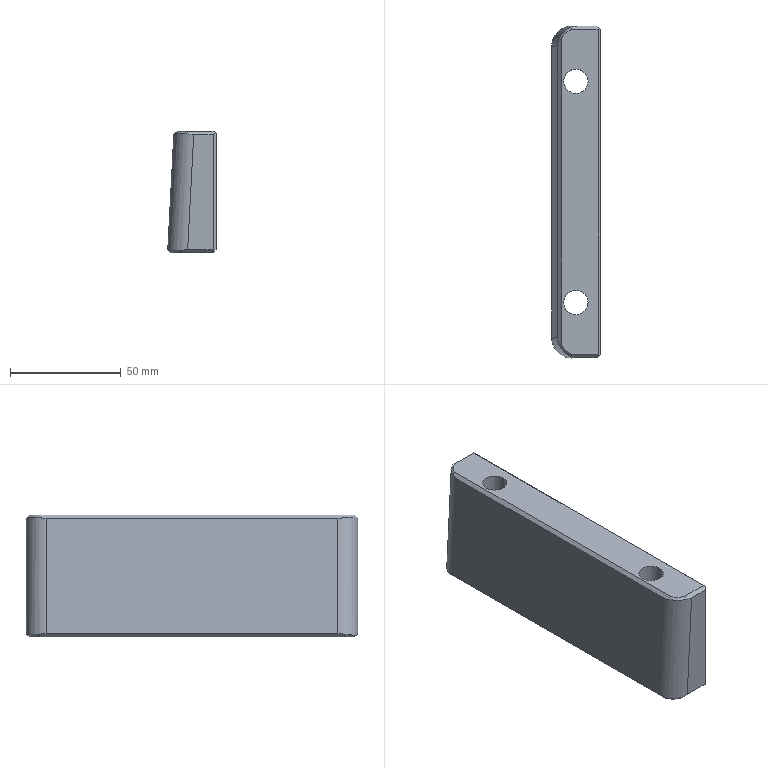Part | Creo | 1 solid | 39 faces | box 21.922 x 150 x 55 mm | volume 149569 mm3 | plane 19 | cylinder 14 | spline 4 | cone 2 | commonest cylinder face diameters 18 x6 11 x4 8.5 x2 10 x2
STEP:
#1=CARTESIAN_POINT('',(-140.,-145.005,33.5));
#2=VERTEX_POINT('',#1);
#3=CARTESIAN_POINT('',(-122.,-145.005,33.5));
#4=VERTEX_POINT('',#3);
#5=CARTESIAN_POINT('',(-131.,-145.005,33.5));
#6=DIRECTION('',(0.,0.,1.));
#7=DIRECTION('',(-1.,-0.000000059,0.));
#8=AXIS2_PLACEMENT_3D('',#5,#6,#7);
#9=CIRCLE('',#8,9.);
#10=EDGE_CURVE('',#2,#4,#9,.T.);
#11=ORIENTED_EDGE('',*,*,#10,.T.);
#12=CARTESIAN_POINT('',(-122.,-145.005,49.5));
#13=VERTEX_POINT('',#12);
#14=CARTESIAN_POINT('',(-122.,-145.005,33.5));
#15=DIRECTION('',(0.,-0.000000011,1.));
#16=VECTOR('',#15,16.);
#17=LINE('',#14,#16);
#18=EDGE_CURVE('',#4,#13,#17,.T.);
#19=ORIENTED_EDGE('',*,*,#18,.T.);
#20=CARTESIAN_POINT('',(-140.,-145.005,49.5));
#21=VERTEX_POINT('',#20);
#22=CARTESIAN_POINT('',(-131.,-145.005,49.5));
#23=DIRECTION('',(0.,0.,-1.));
#24=DIRECTION('',(1.,0.,0.));
#25=AXIS2_PLACEMENT_3D('',#22,#23,#24);
#26=CIRCLE('',#25,9.);
#27=EDGE_CURVE('',#13,#21,#26,.T.);
#28=ORIENTED_EDGE('',*,*,#27,.T.);
#29=CARTESIAN_POINT('',(-140.,-145.005,33.5));
#30=DIRECTION('',(0.,0.,1.));
#31=VECTOR('',#30,16.);
#32=LINE('',#29,#31);
#33=EDGE_CURVE('',#2,#21,#32,.T.);
#34=ORIENTED_EDGE('',*,*,#33,.F.);
#35=EDGE_LOOP('',(#11,#19,#28,#34));
#36=FACE_OUTER_BOUND('',#35,.F.);
#37=CARTESIAN_POINT('',(-131.,-145.005,32.95));
#38=DIRECTION('',(0.,0.,1.));
#39=DIRECTION('',(-1.,-0.000000059,0.));
#40=AXIS2_PLACEMENT_3D('',#37,#38,#39);
#41=CYLINDRICAL_SURFACE('',#40,9.);
#42=ADVANCED_FACE('',(#36),#41,.F.);
#43=CARTESIAN_POINT('',(-140.5,-163.758,33.5));
#44=VERTEX_POINT('',#43);
#45=CARTESIAN_POINT('',(-140.5,-26.251,33.5));
#46=VERTEX_POINT('',#45);
#47=CARTESIAN_POINT('',(-140.5,-163.758,33.5));
#48=DIRECTION('',(-0.000000059,1.,0.));
#49=VECTOR('',#48,137.507);
#50=LINE('',#47,#49);
#51=EDGE_CURVE('',#44,#46,#50,.T.);
#52=ORIENTED_EDGE('',*,*,#51,.F.);
#53=CARTESIAN_POINT('',(-135.628,-168.581,33.5));
#54=VERTEX_POINT('',#53);
#55=CARTESIAN_POINT('',(-135.628,-168.581,33.5));
#56=CARTESIAN_POINT('',(-137.859,-167.798,33.5));
#57=CARTESIAN_POINT('',(-139.697,-165.98,33.5));
#58=CARTESIAN_POINT('',(-140.5,-163.758,33.5));
#59=B_SPLINE_CURVE_WITH_KNOTS('',3,(#55,#56,#57,#58),.UNSPECIFIED.,.F.,.F.,(4,4),(0.,1.),.UNSPECIFIED.);
#60=EDGE_CURVE('',#54,#44,#59,.T.);
#61=ORIENTED_EDGE('',*,*,#60,.F.);
#62=CARTESIAN_POINT('',(-121.423,-168.581,33.5));
#63=VERTEX_POINT('',#62);
#64=CARTESIAN_POINT('',(-121.423,-168.581,33.5));
#65=DIRECTION('',(-1.,-0.000000062,-0.000000002));
#66=VECTOR('',#65,14.205);
#67=LINE('',#64,#66);
#68=EDGE_CURVE('',#63,#54,#67,.T.);
#69=ORIENTED_EDGE('',*,*,#68,.F.);
#70=CARTESIAN_POINT('',(-121.423,-21.428,33.5));
#71=VERTEX_POINT('',#70);
#72=CARTESIAN_POINT('',(-121.423,-21.428,33.5));
#73=DIRECTION('',(0.000000059,-1.,0.));
#74=VECTOR('',#73,147.153);
#75=LINE('',#72,#74);
#76=EDGE_CURVE('',#71,#63,#75,.T.);
#77=ORIENTED_EDGE('',*,*,#76,.F.);
#78=CARTESIAN_POINT('',(-135.628,-21.428,33.5));
#79=VERTEX_POINT('',#78);
#80=CARTESIAN_POINT('',(-135.628,-21.428,33.5));
#81=DIRECTION('',(1.,0.000000059,0.));
#82=VECTOR('',#81,14.205);
#83=LINE('',#80,#82);
#84=EDGE_CURVE('',#79,#71,#83,.T.);
#85=ORIENTED_EDGE('',*,*,#84,.F.);
#86=CARTESIAN_POINT('',(-140.5,-26.251,33.5));
#87=CARTESIAN_POINT('',(-139.697,-24.029,33.5));
#88=CARTESIAN_POINT('',(-137.859,-22.211,33.5));
#89=B_SPLINE_CURVE_WITH_KNOTS('',3,(#86,#87,#88,#78),.UNSPECIFIED.,.F.,.F.,(4,4),(0.,1.),.UNSPECIFIED.);
#90=EDGE_CURVE('',#46,#79,#89,.T.);
#91=ORIENTED_EDGE('',*,*,#90,.F.);
#92=EDGE_LOOP('',(#52,#61,#69,#77,#85,#91));
#93=FACE_OUTER_BOUND('',#92,.F.);
#94=CARTESIAN_POINT('',(-140.,-45.005,33.5));
#95=VERTEX_POINT('',#94);
#96=CARTESIAN_POINT('',(-122.,-45.005,33.5));
#97=VERTEX_POINT('',#96);
#98=CARTESIAN_POINT('',(-131.,-45.005,33.5));
#99=DIRECTION('',(0.,0.,1.));
#100=DIRECTION('',(-1.,-0.000000059,0.));
#101=AXIS2_PLACEMENT_3D('',#98,#99,#100);
#102=CIRCLE('',#101,9.);
#103=EDGE_CURVE('',#95,#97,#102,.T.);
#104=ORIENTED_EDGE('',*,*,#103,.F.);
#105=CARTESIAN_POINT('',(-131.,-45.005,33.5));
#106=DIRECTION('',(0.,0.,1.));
#107=DIRECTION('',(1.,0.000000059,0.));
#108=AXIS2_PLACEMENT_3D('',#105,#106,#107);
#109=CIRCLE('',#108,9.);
#110=EDGE_CURVE('',#97,#95,#109,.T.);
#111=ORIENTED_EDGE('',*,*,#110,.F.);
#112=EDGE_LOOP('',(#104,#111));
#113=FACE_BOUND('',#112,.F.);
#114=ORIENTED_EDGE('',*,*,#10,.F.);
#115=CARTESIAN_POINT('',(-131.,-145.005,33.5));
#116=DIRECTION('',(0.,0.,1.));
#117=DIRECTION('',(1.,0.000000059,0.));
#118=AXIS2_PLACEMENT_3D('',#115,#116,#117);
#119=CIRCLE('',#118,9.);
#120=EDGE_CURVE('',#4,#2,#119,.T.);
#121=ORIENTED_EDGE('',*,*,#120,.F.);
#122=EDGE_LOOP('',(#114,#121));
#123=FACE_BOUND('',#122,.F.);
#124=CARTESIAN_POINT('',(-126.,-95.005,33.5));
#125=VERTEX_POINT('',#124);
#126=CARTESIAN_POINT('',(-136.,-95.005,33.5));
#127=VERTEX_POINT('',#126);
#128=CARTESIAN_POINT('',(-131.,-95.005,33.5));
#129=DIRECTION('',(0.,0.,1.));
#130=DIRECTION('',(1.,0.,0.));
#131=AXIS2_PLACEMENT_3D('',#128,#129,#130);
#132=CIRCLE('',#131,5.);
#133=EDGE_CURVE('',#125,#127,#132,.T.);
#134=ORIENTED_EDGE('',*,*,#133,.F.);
#135=CARTESIAN_POINT('',(-131.,-95.005,33.5));
#136=DIRECTION('',(0.,0.,1.));
#137=DIRECTION('',(-1.,0.,0.));
#138=AXIS2_PLACEMENT_3D('',#135,#136,#137);
#139=CIRCLE('',#138,5.);
#140=EDGE_CURVE('',#127,#125,#139,.T.);
#141=ORIENTED_EDGE('',*,*,#140,.F.);
#142=EDGE_LOOP('',(#134,#141));
#143=FACE_BOUND('',#142,.F.);
#144=CARTESIAN_POINT('',(-142.,-20.005,33.5));
#145=DIRECTION('',(0.,0.,-1.));
#146=DIRECTION('',(1.,0.000000059,0.));
#147=AXIS2_PLACEMENT_3D('',#144,#145,#146);
#148=PLANE('',#147);
#149=ADVANCED_FACE('',(#93,#113,#123,#143),#148,.T.);
#150=ORIENTED_EDGE('',*,*,#120,.T.);
#151=ORIENTED_EDGE('',*,*,#33,.T.);
#152=CARTESIAN_POINT('',(-131.,-145.005,49.5));
#153=DIRECTION('',(0.,0.,-1.));
#154=DIRECTION('',(-1.,-0.000000059,0.));
#155=AXIS2_PLACEMENT_3D('',#152,#153,#154);
#156=CIRCLE('',#155,9.);
#157=EDGE_CURVE('',#21,#13,#156,.T.);
#158=ORIENTED_EDGE('',*,*,#157,.T.);
#159=ORIENTED_EDGE('',*,*,#18,.F.);
#160=EDGE_LOOP('',(#150,#151,#158,#159));
#161=FACE_OUTER_BOUND('',#160,.F.);
#162=CARTESIAN_POINT('',(-131.,-145.005,32.95));
#163=DIRECTION('',(0.,0.,1.));
#164=DIRECTION('',(-1.,-0.000000059,0.));
#165=AXIS2_PLACEMENT_3D('',#162,#163,#164);
#166=CYLINDRICAL_SURFACE('',#165,9.);
#167=ADVANCED_FACE('',(#161),#166,.F.);
#168=ORIENTED_EDGE('',*,*,#27,.F.);
#169=ORIENTED_EDGE('',*,*,#157,.F.);
#170=EDGE_LOOP('',(#168,#169));
#171=FACE_OUTER_BOUND('',#170,.F.);
#172=CARTESIAN_POINT('',(-125.5,-145.005,49.5));
#173=VERTEX_POINT('',#172);
#174=CARTESIAN_POINT('',(-136.5,-145.005,49.5));
#175=VERTEX_POINT('',#174);
#176=CARTESIAN_POINT('',(-131.,-145.005,49.5));
#177=DIRECTION('',(0.,0.,1.));
#178=DIRECTION('',(1.,0.,0.));
#179=AXIS2_PLACEMENT_3D('',#176,#177,#178);
#180=CIRCLE('',#179,5.5);
#181=EDGE_CURVE('',#173,#175,#180,.T.);
#182=ORIENTED_EDGE('',*,*,#181,.F.);
#183=CARTESIAN_POINT('',(-131.,-145.005,49.5));
#184=DIRECTION('',(0.,0.,1.));
#185=DIRECTION('',(-1.,-0.000000059,0.));
#186=AXIS2_PLACEMENT_3D('',#183,#184,#185);
#187=CIRCLE('',#186,5.5);
#188=EDGE_CURVE('',#175,#173,#187,.T.);
#189=ORIENTED_EDGE('',*,*,#188,.F.);
#190=EDGE_LOOP('',(#182,#189));
#191=FACE_BOUND('',#190,.F.);
#192=CARTESIAN_POINT('',(-131.,-145.005,49.5));
#193=DIRECTION('',(0.,0.,1.));
#194=DIRECTION('',(-1.,-0.000000059,0.));
#195=AXIS2_PLACEMENT_3D('',#192,#193,#194);
#196=PLANE('',#195);
#197=ADVANCED_FACE('',(#171,#191),#196,.F.);
#198=ORIENTED_EDGE('',*,*,#181,.T.);
#199=CARTESIAN_POINT('',(-136.5,-145.005,88.5));
#200=VERTEX_POINT('',#199);
#201=CARTESIAN_POINT('',(-136.5,-145.005,88.5));
#202=DIRECTION('',(0.,0.,-1.));
#203=VECTOR('',#202,39.);
#204=LINE('',#201,#203);
#205=EDGE_CURVE('',#200,#175,#204,.T.);
#206=ORIENTED_EDGE('',*,*,#205,.F.);
#207=CARTESIAN_POINT('',(-125.5,-145.005,88.5));
#208=VERTEX_POINT('',#207);
#209=CARTESIAN_POINT('',(-131.,-145.005,88.5));
#210=DIRECTION('',(0.,0.,-1.));
#211=DIRECTION('',(-1.,-0.000000059,0.));
#212=AXIS2_PLACEMENT_3D('',#209,#210,#211);
#213=CIRCLE('',#212,5.5);
#214=EDGE_CURVE('',#200,#208,#213,.T.);
#215=ORIENTED_EDGE('',*,*,#214,.T.);
#216=CARTESIAN_POINT('',(-125.5,-145.005,88.5));
#217=DIRECTION('',(0.,-0.000000003,-1.));
#218=VECTOR('',#217,39.);
#219=LINE('',#216,#218);
#220=EDGE_CURVE('',#208,#173,#219,.T.);
#221=ORIENTED_EDGE('',*,*,#220,.T.);
#222=EDGE_LOOP('',(#198,#206,#215,#221));
#223=FACE_OUTER_BOUND('',#222,.F.);
#224=CARTESIAN_POINT('',(-131.,-145.005,44.5));
#225=DIRECTION('',(0.,0.,-1.));
#226=DIRECTION('',(-1.,-0.000000059,0.));
#227=AXIS2_PLACEMENT_3D('',#224,#225,#226);
#228=CYLINDRICAL_SURFACE('',#227,5.5);
#229=ADVANCED_FACE('',(#223),#228,.F.);
#230=ORIENTED_EDGE('',*,*,#188,.T.);
#231=ORIENTED_EDGE('',*,*,#220,.F.);
#232=CARTESIAN_POINT('',(-131.,-145.005,88.5));
#233=DIRECTION('',(0.,0.,-1.));
#234=DIRECTION('',(1.,0.000000059,0.));
#235=AXIS2_PLACEMENT_3D('',#232,#233,#234);
#236=CIRCLE('',#235,5.5);
#237=EDGE_CURVE('',#208,#200,#236,.T.);
#238=ORIENTED_EDGE('',*,*,#237,.T.);
#239=ORIENTED_EDGE('',*,*,#205,.T.);
#240=EDGE_LOOP('',(#230,#231,#238,#239));
#241=FACE_OUTER_BOUND('',#240,.F.);
#242=CARTESIAN_POINT('',(-131.,-145.005,44.5));
#243=DIRECTION('',(0.,0.,-1.));
#244=DIRECTION('',(-1.,-0.000000059,0.));
#245=AXIS2_PLACEMENT_3D('',#242,#243,#244);
#246=CYLINDRICAL_SURFACE('',#245,5.5);
#247=ADVANCED_FACE('',(#241),#246,.F.);
#248=CARTESIAN_POINT('',(-121.,-21.585,88.5));
#249=VERTEX_POINT('',#248);
#250=CARTESIAN_POINT('',(-133.06,-21.585,88.5));
#251=VERTEX_POINT('',#250);
#252=CARTESIAN_POINT('',(-121.,-21.585,88.5));
#253=DIRECTION('',(-1.,-0.000000052,0.000000002));
#254=VECTOR('',#253,12.06);
#255=LINE('',#252,#254);
#256=EDGE_CURVE('',#249,#251,#255,.T.);
#257=ORIENTED_EDGE('',*,*,#256,.F.);
#258=CARTESIAN_POINT('',(-121.,-168.424,88.5));
#259=VERTEX_POINT('',#258);
#260=CARTESIAN_POINT('',(-121.,-21.585,88.5));
#261=DIRECTION('',(0.000000059,-1.,0.));
#262=VECTOR('',#261,146.839);
#263=LINE('',#260,#262);
#264=EDGE_CURVE('',#249,#259,#263,.T.);
#265=ORIENTED_EDGE('',*,*,#264,.T.);
#266=CARTESIAN_POINT('',(-133.06,-168.424,88.5));
#267=VERTEX_POINT('',#266);
#268=CARTESIAN_POINT('',(-133.06,-168.424,88.5));
#269=DIRECTION('',(1.,0.000000059,0.));
#270=VECTOR('',#269,12.06);
#271=LINE('',#268,#270);
#272=EDGE_CURVE('',#267,#259,#271,.T.);
#273=ORIENTED_EDGE('',*,*,#272,.F.);
#274=CARTESIAN_POINT('',(-137.618,-163.828,88.5));
#275=VERTEX_POINT('',#274);
#276=CARTESIAN_POINT('',(-137.618,-163.828,88.5));
#277=CARTESIAN_POINT('',(-136.834,-165.908,88.5));
#278=CARTESIAN_POINT('',(-135.136,-167.622,88.5));
#279=B_SPLINE_CURVE_WITH_KNOTS('',3,(#276,#277,#278,#266),.UNSPECIFIED.,.F.,.F.,(4,4),(0.,1.),.UNSPECIFIED.);
#280=EDGE_CURVE('',#275,#267,#279,.T.);
#281=ORIENTED_EDGE('',*,*,#280,.F.);
#282=CARTESIAN_POINT('',(-137.618,-26.182,88.5));
#283=VERTEX_POINT('',#282);
#284=CARTESIAN_POINT('',(-137.618,-26.182,88.5));
#285=DIRECTION('',(0.000000058,-1.,0.));
#286=VECTOR('',#285,137.646);
#287=LINE('',#284,#286);
#288=EDGE_CURVE('',#283,#275,#287,.T.);
#289=ORIENTED_EDGE('',*,*,#288,.F.);
#290=CARTESIAN_POINT('',(-133.06,-21.585,88.5));
#291=CARTESIAN_POINT('',(-135.136,-22.388,88.5));
#292=CARTESIAN_POINT('',(-136.834,-24.101,88.5));
#293=B_SPLINE_CURVE_WITH_KNOTS('',3,(#290,#291,#292,#282),.UNSPECIFIED.,.F.,.F.,(4,4),(0.,1.),.UNSPECIFIED.);
#294=EDGE_CURVE('',#251,#283,#293,.T.);
#295=ORIENTED_EDGE('',*,*,#294,.F.);
#296=EDGE_LOOP('',(#257,#265,#273,#281,#289,#295));
#297=FACE_OUTER_BOUND('',#296,.F.);
#298=CARTESIAN_POINT('',(-136.5,-45.005,88.5));
#299=VERTEX_POINT('',#298);
#300=CARTESIAN_POINT('',(-125.5,-45.005,88.5));
#301=VERTEX_POINT('',#300);
#302=CARTESIAN_POINT('',(-131.,-45.005,88.5));
#303=DIRECTION('',(0.,0.,-1.));
#304=DIRECTION('',(-1.,-0.000000059,0.));
#305=AXIS2_PLACEMENT_3D('',#302,#303,#304);
#306=CIRCLE('',#305,5.5);
#307=EDGE_CURVE('',#299,#301,#306,.T.);
#308=ORIENTED_EDGE('',*,*,#307,.F.);
#309=CARTESIAN_POINT('',(-131.,-45.005,88.5));
#310=DIRECTION('',(0.,0.,-1.));
#311=DIRECTION('',(1.,0.000000059,0.));
#312=AXIS2_PLACEMENT_3D('',#309,#310,#311);
#313=CIRCLE('',#312,5.5);
#314=EDGE_CURVE('',#301,#299,#313,.T.);
#315=ORIENTED_EDGE('',*,*,#314,.F.);
#316=EDGE_LOOP('',(#308,#315));
#317=FACE_BOUND('',#316,.F.);
#318=ORIENTED_EDGE('',*,*,#214,.F.);
#319=ORIENTED_EDGE('',*,*,#237,.F.);
#320=EDGE_LOOP('',(#318,#319));
#321=FACE_BOUND('',#320,.F.);
#322=CARTESIAN_POINT('',(-120.,-20.005,88.5));
#323=DIRECTION('',(0.,0.,1.));
#324=DIRECTION('',(-1.,-0.000000059,0.));
#325=AXIS2_PLACEMENT_3D('',#322,#323,#324);
#326=PLANE('',#325);
#327=ADVANCED_FACE('',(#297,#317,#321),#326,.T.);
#328=CARTESIAN_POINT('',(-125.5,-45.005,49.5));
#329=VERTEX_POINT('',#328);
#330=CARTESIAN_POINT('',(-136.5,-45.005,49.5));
#331=VERTEX_POINT('',#330);
#332=CARTESIAN_POINT('',(-131.,-45.005,49.5));
#333=DIRECTION('',(0.,0.,1.));
#334=DIRECTION('',(1.,0.,0.));
#335=AXIS2_PLACEMENT_3D('',#332,#333,#334);
#336=CIRCLE('',#335,5.5);
#337=EDGE_CURVE('',#329,#331,#336,.T.);
#338=ORIENTED_EDGE('',*,*,#337,.T.);
#339=CARTESIAN_POINT('',(-136.5,-45.005,88.5));
#340=DIRECTION('',(0.,0.,-1.));
#341=VECTOR('',#340,39.);
#342=LINE('',#339,#341);
#343=EDGE_CURVE('',#299,#331,#342,.T.);
#344=ORIENTED_EDGE('',*,*,#343,.F.);
#345=ORIENTED_EDGE('',*,*,#307,.T.);
#346=CARTESIAN_POINT('',(-125.5,-45.005,88.5));
#347=DIRECTION('',(0.,-0.000000003,-1.));
#348=VECTOR('',#347,39.);
#349=LINE('',#346,#348);
#350=EDGE_CURVE('',#301,#329,#349,.T.);
#351=ORIENTED_EDGE('',*,*,#350,.T.);
#352=EDGE_LOOP('',(#338,#344,#345,#351));
#353=FACE_OUTER_BOUND('',#352,.F.);
#354=CARTESIAN_POINT('',(-131.,-45.005,44.5));
#355=DIRECTION('',(0.,0.,-1.));
#356=DIRECTION('',(-1.,-0.000000059,0.));
#357=AXIS2_PLACEMENT_3D('',#354,#355,#356);
#358=CYLINDRICAL_SURFACE('',#357,5.5);
#359=ADVANCED_FACE('',(#353),#358,.F.);
#360=CARTESIAN_POINT('',(-122.,-45.005,49.5));
#361=VERTEX_POINT('',#360);
#362=CARTESIAN_POINT('',(-140.,-45.005,49.5));
#363=VERTEX_POINT('',#362);
#364=CARTESIAN_POINT('',(-131.,-45.005,49.5));
#365=DIRECTION('',(0.,0.,-1.));
#366=DIRECTION('',(1.,0.,0.));
#367=AXIS2_PLACEMENT_3D('',#364,#365,#366);
#368=CIRCLE('',#367,9.);
#369=EDGE_CURVE('',#361,#363,#368,.T.);
#370=ORIENTED_EDGE('',*,*,#369,.F.);
#371=CARTESIAN_POINT('',(-131.,-45.005,49.5));
#372=DIRECTION('',(0.,0.,-1.));
#373=DIRECTION('',(-1.,-0.000000059,0.));
#374=AXIS2_PLACEMENT_3D('',#371,#372,#373);
#375=CIRCLE('',#374,9.);
#376=EDGE_CURVE('',#363,#361,#375,.T.);
#377=ORIENTED_EDGE('',*,*,#376,.F.);
#378=EDGE_LOOP('',(#370,#377));
#379=FACE_OUTER_BOUND('',#378,.F.);
#380=ORIENTED_EDGE('',*,*,#337,.F.);
#381=CARTESIAN_POINT('',(-131.,-45.005,49.5));
#382=DIRECTION('',(0.,0.,1.));
#383=DIRECTION('',(-1.,-0.000000059,0.));
#384=AXIS2_PLACEMENT_3D('',#381,#382,#383);
#385=CIRCLE('',#384,5.5);
#386=EDGE_CURVE('',#331,#329,#385,.T.);
#387=ORIENTED_EDGE('',*,*,#386,.F.);
#388=EDGE_LOOP('',(#380,#387));
#389=FACE_BOUND('',#388,.F.);
#390=CARTESIAN_POINT('',(-131.,-45.005,49.5));
#391=DIRECTION('',(0.,0.,1.));
#392=DIRECTION('',(-1.,-0.000000059,0.));
#393=AXIS2_PLACEMENT_3D('',#390,#391,#392);
#394=PLANE('',#393);
#395=ADVANCED_FACE('',(#379,#389),#394,.F.);
#396=ORIENTED_EDGE('',*,*,#386,.T.);
#397=ORIENTED_EDGE('',*,*,#350,.F.);
#398=ORIENTED_EDGE('',*,*,#314,.T.);
#399=ORIENTED_EDGE('',*,*,#343,.T.);
#400=EDGE_LOOP('',(#396,#397,#398,#399));
#401=FACE_OUTER_BOUND('',#400,.F.);
#402=CARTESIAN_POINT('',(-131.,-45.005,44.5));
#403=DIRECTION('',(0.,0.,-1.));
#404=DIRECTION('',(-1.,-0.000000059,0.));
#405=AXIS2_PLACEMENT_3D('',#402,#403,#404);
#406=CYLINDRICAL_SURFACE('',#405,5.5);
#407=ADVANCED_FACE('',(#401),#406,.F.);
#408=ORIENTED_EDGE('',*,*,#103,.T.);
#409=CARTESIAN_POINT('',(-122.,-45.005,33.5));
#410=DIRECTION('',(0.,-0.000000011,1.));
#411=VECTOR('',#410,16.);
#412=LINE('',#409,#411);
#413=EDGE_CURVE('',#97,#361,#412,.T.);
#414=ORIENTED_EDGE('',*,*,#413,.T.);
#415=ORIENTED_EDGE('',*,*,#369,.T.);
#416=CARTESIAN_POINT('',(-140.,-45.005,33.5));
#417=DIRECTION('',(0.,0.,1.));
#418=VECTOR('',#417,16.);
#419=LINE('',#416,#418);
#420=EDGE_CURVE('',#95,#363,#419,.T.);
#421=ORIENTED_EDGE('',*,*,#420,.F.);
#422=EDGE_LOOP('',(#408,#414,#415,#421));
#423=FACE_OUTER_BOUND('',#422,.F.);
#424=CARTESIAN_POINT('',(-131.,-45.005,32.95));
#425=DIRECTION('',(0.,0.,1.));
#426=DIRECTION('',(-1.,-0.000000059,0.));
#427=AXIS2_PLACEMENT_3D('',#424,#425,#426);
#428=CYLINDRICAL_SURFACE('',#427,9.);
#429=ADVANCED_FACE('',(#423),#428,.F.);
#430=ORIENTED_EDGE('',*,*,#110,.T.);
#431=ORIENTED_EDGE('',*,*,#420,.T.);
#432=ORIENTED_EDGE('',*,*,#376,.T.);
#433=ORIENTED_EDGE('',*,*,#413,.F.);
#434=EDGE_LOOP('',(#430,#431,#432,#433));
#435=FACE_OUTER_BOUND('',#434,.F.);
#436=CARTESIAN_POINT('',(-131.,-45.005,32.95));
#437=DIRECTION('',(0.,0.,1.));
#438=DIRECTION('',(-1.,-0.000000059,0.));
#439=AXIS2_PLACEMENT_3D('',#436,#437,#438);
#440=CYLINDRICAL_SURFACE('',#439,9.);
#441=ADVANCED_FACE('',(#435),#440,.F.);
#442=CARTESIAN_POINT('',(-130.658,-20.017,86.932));
#443=VERTEX_POINT('',#442);
#444=CARTESIAN_POINT('',(-130.188,-20.005,86.919));
#445=VERTEX_POINT('',#444);
#446=CARTESIAN_POINT('',(-130.502,-20.009,86.923));
#447=CARTESIAN_POINT('',(-130.345,-20.005,86.919));
#448=B_SPLINE_CURVE_WITH_KNOTS('',3,(#442,#446,#447,#444),.UNSPECIFIED.,.F.,.F.,(4,4),(0.,1.),.UNSPECIFIED.);
#449=EDGE_CURVE('',#443,#445,#448,.T.);
#450=ORIENTED_EDGE('',*,*,#449,.T.);
#451=CARTESIAN_POINT('',(-121.423,-20.005,86.919));
#452=VERTEX_POINT('',#451);
#453=CARTESIAN_POINT('',(-121.423,-20.005,86.919));
#454=DIRECTION('',(-1.,-0.000000059,0.));
#455=VECTOR('',#454,8.765);
#456=LINE('',#453,#455);
#457=EDGE_CURVE('',#452,#445,#456,.T.);
#458=ORIENTED_EDGE('',*,*,#457,.F.);
#459=CARTESIAN_POINT('',(-120.421,-21.007,87.921));
#460=VERTEX_POINT('',#459);
#461=CARTESIAN_POINT('',(-121.423,-20.005,86.919));
#462=DIRECTION('',(0.5774,-0.5774,0.5774));
#463=VECTOR('',#462,1.736);
#464=LINE('',#461,#463);
#465=EDGE_CURVE('',#452,#460,#464,.T.);
#466=ORIENTED_EDGE('',*,*,#465,.T.);
#467=CARTESIAN_POINT('',(-120.421,-21.007,87.921));
#468=DIRECTION('',(-0.5774,-0.5774,0.5774));
#469=VECTOR('',#468,1.002);
#470=LINE('',#467,#469);
#471=EDGE_CURVE('',#460,#249,#470,.T.);
#472=ORIENTED_EDGE('',*,*,#471,.T.);
#473=ORIENTED_EDGE('',*,*,#256,.T.);
#474=CARTESIAN_POINT('',(-133.299,-20.569,87.483));
#475=VERTEX_POINT('',#474);
#476=CARTESIAN_POINT('',(-133.06,-21.585,88.5));
#477=CARTESIAN_POINT('',(-133.087,-21.474,88.388));
#478=CARTESIAN_POINT('',(-133.141,-21.249,88.164));
#479=CARTESIAN_POINT('',(-133.22,-20.91,87.825));
#480=CARTESIAN_POINT('',(-133.273,-20.683,87.598));
#481=CARTESIAN_POINT('',(-133.299,-20.569,87.483));
#482=B_SPLINE_CURVE_WITH_KNOTS('',3,(#476,#477,#478,#479,#480,#481),.UNSPECIFIED.,.F.,.F.,(4,1,1,4),(0.,0.3333,0.6667,1.),.UNSPECIFIED.);
#483=EDGE_CURVE('',#251,#475,#482,.T.);
#484=ORIENTED_EDGE('',*,*,#483,.T.);
#485=CARTESIAN_POINT('',(-133.013,-20.461,87.375));
#486=CARTESIAN_POINT('',(-132.436,-20.277,87.191));
#487=CARTESIAN_POINT('',(-131.55,-20.093,87.008));
#488=CARTESIAN_POINT('',(-130.956,-20.033,86.947));
#489=CARTESIAN_POINT('',(-130.658,-20.017,86.932));
#490=B_SPLINE_CURVE_WITH_KNOTS('',3,(#474,#485,#486,#487,#488,#489),.UNSPECIFIED.,.F.,.F.,(4,1,1,4),(0.,0.3333,0.6667,1.),.UNSPECIFIED.);
#491=EDGE_CURVE('',#475,#443,#490,.T.);
#492=ORIENTED_EDGE('',*,*,#491,.T.);
#493=EDGE_LOOP('',(#450,#458,#466,#472,#473,#484,#492));
#494=FACE_OUTER_BOUND('',#493,.F.);
#495=CARTESIAN_POINT('',(-125.595,-20.795,87.71));
#496=DIRECTION('',(-0.000000042,0.7071,0.7071));
#497=DIRECTION('',(0.000000042,-0.7071,0.7071));
#498=AXIS2_PLACEMENT_3D('',#495,#496,#497);
#499=PLANE('',#498);
#500=ADVANCED_FACE('',(#494),#499,.T.);
#501=CARTESIAN_POINT('',(-132.913,-20.005,34.923));
#502=VERTEX_POINT('',#501);
#503=CARTESIAN_POINT('',(-135.739,-20.451,34.477));
#504=VERTEX_POINT('',#503);
#505=CARTESIAN_POINT('',(-133.222,-20.005,34.923));
#506=CARTESIAN_POINT('',(-133.844,-20.036,34.892));
#507=CARTESIAN_POINT('',(-134.794,-20.184,34.745));
#508=CARTESIAN_POINT('',(-135.424,-20.35,34.578));
#509=CARTESIAN_POINT('',(-135.739,-20.451,34.477));
#510=B_SPLINE_CURVE_WITH_KNOTS('',3,(#501,#505,#506,#507,#508,#509),.UNSPECIFIED.,.F.,.F.,(4,1,1,4),(0.,0.3333,0.6667,1.),.UNSPECIFIED.);
#511=EDGE_CURVE('',#502,#504,#510,.T.);
#512=ORIENTED_EDGE('',*,*,#511,.F.);
#513=CARTESIAN_POINT('',(-132.913,-20.005,34.923));
#514=DIRECTION('',(0.05234,0.000000003,0.9986));
#515=VECTOR('',#514,52.067);
#516=LINE('',#513,#515);
#517=EDGE_CURVE('',#502,#445,#516,.T.);
#518=ORIENTED_EDGE('',*,*,#517,.T.);
#519=ORIENTED_EDGE('',*,*,#449,.F.);
#520=ORIENTED_EDGE('',*,*,#491,.F.);
#521=CARTESIAN_POINT('',(-138.655,-26.008,87.516));
#522=VERTEX_POINT('',#521);
#523=CARTESIAN_POINT('',(-133.299,-20.569,87.483));
#524=CARTESIAN_POINT('',(-133.795,-20.753,87.489));
#525=CARTESIAN_POINT('',(-134.752,-21.208,87.497));
#526=CARTESIAN_POINT('',(-136.037,-22.124,87.505));
#527=CARTESIAN_POINT('',(-137.144,-23.248,87.512));
#528=CARTESIAN_POINT('',(-138.039,-24.547,87.516));
#529=CARTESIAN_POINT('',(-138.479,-25.51,87.517));
#530=CARTESIAN_POINT('',(-138.655,-26.008,87.516));
#531=B_SPLINE_CURVE_WITH_KNOTS('',3,(#523,#524,#525,#526,#527,#528,#529,#530),.UNSPECIFIED.,.F.,.F.,(4,1,1,1,1,4),(0.,0.2,0.4,0.6,0.8,1.),.UNSPECIFIED.);
#532=EDGE_CURVE('',#475,#522,#531,.T.);
#533=ORIENTED_EDGE('',*,*,#532,.T.);
#534=CARTESIAN_POINT('',(-139.196,-29.005,87.002));
#535=VERTEX_POINT('',#534);
#536=CARTESIAN_POINT('',(-139.196,-28.672,87.002));
#537=CARTESIAN_POINT('',(-139.158,-28.007,87.038));
#538=CARTESIAN_POINT('',(-138.979,-26.999,87.208));
#539=CARTESIAN_POINT('',(-138.777,-26.337,87.4));
#540=CARTESIAN_POINT('',(-138.655,-26.008,87.516));
#541=B_SPLINE_CURVE_WITH_KNOTS('',3,(#534,#536,#537,#538,#539,#540),.UNSPECIFIED.,.F.,.F.,(4,1,1,4),(0.,0.3333,0.6667,1.),.UNSPECIFIED.);
#542=EDGE_CURVE('',#535,#522,#541,.T.);
#543=ORIENTED_EDGE('',*,*,#542,.F.);
#544=CARTESIAN_POINT('',(-141.921,-29.005,34.998));
#545=VERTEX_POINT('',#544);
#546=CARTESIAN_POINT('',(-141.921,-29.005,34.998));
#547=DIRECTION('',(0.05234,0.000000006,0.9986));
#548=VECTOR('',#547,52.075);
#549=LINE('',#546,#548);
#550=EDGE_CURVE('',#545,#535,#549,.T.);
#551=ORIENTED_EDGE('',*,*,#550,.F.);
#552=CARTESIAN_POINT('',(-141.458,-26.079,34.509));
#553=VERTEX_POINT('',#552);
#554=CARTESIAN_POINT('',(-141.562,-26.4,34.619));
#555=CARTESIAN_POINT('',(-141.734,-27.044,34.801));
#556=CARTESIAN_POINT('',(-141.888,-28.028,34.963));
#557=CARTESIAN_POINT('',(-141.921,-28.679,34.998));
#558=CARTESIAN_POINT('',(-141.921,-29.005,34.998));
#559=B_SPLINE_CURVE_WITH_KNOTS('',3,(#552,#554,#555,#556,#557,#558),.UNSPECIFIED.,.F.,.F.,(4,1,1,4),(0.,0.3333,0.6667,1.),.UNSPECIFIED.);
#560=EDGE_CURVE('',#553,#545,#559,.T.);
#561=ORIENTED_EDGE('',*,*,#560,.F.);
#562=CARTESIAN_POINT('',(-141.458,-26.079,34.509));
#563=CARTESIAN_POINT('',(-141.358,-25.789,34.507));
#564=CARTESIAN_POINT('',(-141.128,-25.218,34.505));
#565=CARTESIAN_POINT('',(-140.697,-24.401,34.506));
#566=CARTESIAN_POINT('',(-140.185,-23.632,34.506));
#567=CARTESIAN_POINT('',(-139.595,-22.918,34.505));
#568=CARTESIAN_POINT('',(-138.935,-22.268,34.501));
#569=CARTESIAN_POINT('',(-138.212,-21.689,34.495));
#570=CARTESIAN_POINT('',(-137.434,-21.187,34.487));
#571=CARTESIAN_POINT('',(-136.608,-20.768,34.48));
#572=CARTESIAN_POINT('',(-136.032,-20.547,34.477));
#573=CARTESIAN_POINT('',(-135.739,-20.451,34.477));
#574=B_SPLINE_CURVE_WITH_KNOTS('',3,(#562,#563,#564,#565,#566,#567,#568,#569,#570,#571,#572,#573),.UNSPECIFIED.,.F.,.F.,(4,1,1,1,1,1,1,1,1,4),(0.,0.1111,0.2222,0.3333,0.4444,0.5556,0.6667,0.7778,0.8889,1.),.UNSPECIFIED.);
#575=EDGE_CURVE('',#553,#504,#574,.T.);
#576=ORIENTED_EDGE('',*,*,#575,.T.);
#577=EDGE_LOOP('',(#512,#518,#519,#520,#533,#543,#551,#561,#576));
#578=FACE_OUTER_BOUND('',#577,.F.);
#579=CARTESIAN_POINT('',(-130.13,-29.005,88.029));
#580=DIRECTION('',(0.05234,0.000000003,0.9986));
#581=DIRECTION('',(0.9986,0.,-0.05234));
#582=AXIS2_PLACEMENT_3D('',#579,#580,#581);
#583=CYLINDRICAL_SURFACE('',#582,9.);
#584=ADVANCED_FACE('',(#578),#583,.T.);
#585=ORIENTED_EDGE('',*,*,#84,.T.);
#586=CARTESIAN_POINT('',(-120.712,-20.716,34.212));
#587=VERTEX_POINT('',#586);
#588=CARTESIAN_POINT('',(-120.712,-20.716,34.212));
#589=DIRECTION('',(-0.5774,-0.5774,-0.5774));
#590=VECTOR('',#589,1.233);
#591=LINE('',#588,#590);
#592=EDGE_CURVE('',#587,#71,#591,.T.);
#593=ORIENTED_EDGE('',*,*,#592,.F.);
#594=CARTESIAN_POINT('',(-121.423,-20.005,34.923));
#595=VERTEX_POINT('',#594);
#596=CARTESIAN_POINT('',(-121.423,-20.005,34.923));
#597=DIRECTION('',(0.5774,-0.5774,-0.5774));
#598=VECTOR('',#597,1.233);
#599=LINE('',#596,#598);
#600=EDGE_CURVE('',#595,#587,#599,.T.);
#601=ORIENTED_EDGE('',*,*,#600,.F.);
#602=CARTESIAN_POINT('',(-132.913,-20.005,34.923));
#603=DIRECTION('',(1.,0.000000059,0.));
#604=VECTOR('',#603,11.49);
#605=LINE('',#602,#604);
#606=EDGE_CURVE('',#502,#595,#605,.T.);
#607=ORIENTED_EDGE('',*,*,#606,.F.);
#608=ORIENTED_EDGE('',*,*,#511,.T.);
#609=CARTESIAN_POINT('',(-135.727,-20.561,34.367));
#610=CARTESIAN_POINT('',(-135.703,-20.78,34.148));
#611=CARTESIAN_POINT('',(-135.666,-21.106,33.822));
#612=CARTESIAN_POINT('',(-135.641,-21.321,33.607));
#613=CARTESIAN_POINT('',(-135.628,-21.428,33.5));
#614=B_SPLINE_CURVE_WITH_KNOTS('',3,(#503,#609,#610,#611,#612,#613),.UNSPECIFIED.,.F.,.F.,(4,1,1,4),(0.,0.3333,0.6667,1.),.UNSPECIFIED.);
#615=EDGE_CURVE('',#504,#79,#614,.T.);
#616=ORIENTED_EDGE('',*,*,#615,.T.);
#617=EDGE_LOOP('',(#585,#593,#601,#607,#608,#616));
#618=FACE_OUTER_BOUND('',#617,.F.);
#619=CARTESIAN_POINT('',(-126.957,-20.716,34.212));
#620=DIRECTION('',(-0.000000042,0.7071,-0.7071));
#621=DIRECTION('',(0.000000042,-0.7071,-0.7071));
#622=AXIS2_PLACEMENT_3D('',#619,#620,#621);
#623=PLANE('',#622);
#624=ADVANCED_FACE('',(#618),#623,.T.);
#625=CARTESIAN_POINT('',(-120.,-168.581,34.923));
#626=VERTEX_POINT('',#625);
#627=CARTESIAN_POINT('',(-120.712,-169.293,34.212));
#628=VERTEX_POINT('',#627);
#629=CARTESIAN_POINT('',(-120.,-168.581,34.923));
#630=DIRECTION('',(-0.5774,-0.5774,-0.5774));
#631=VECTOR('',#630,1.233);
#632=LINE('',#629,#631);
#633=EDGE_CURVE('',#626,#628,#632,.T.);
#634=ORIENTED_EDGE('',*,*,#633,.F.);
#635=CARTESIAN_POINT('',(-120.,-21.428,34.923));
#636=VERTEX_POINT('',#635);
#637=CARTESIAN_POINT('',(-120.,-21.428,34.923));
#638=DIRECTION('',(0.000000059,-1.,0.));
#639=VECTOR('',#638,147.153);
#640=LINE('',#637,#639);
#641=EDGE_CURVE('',#636,#626,#640,.T.);
#642=ORIENTED_EDGE('',*,*,#641,.F.);
#643=CARTESIAN_POINT('',(-120.,-21.428,34.923));
#644=DIRECTION('',(-0.5774,0.5774,-0.5774));
#645=VECTOR('',#644,1.233);
#646=LINE('',#643,#645);
#647=EDGE_CURVE('',#636,#587,#646,.T.);
#648=ORIENTED_EDGE('',*,*,#647,.T.);
#649=ORIENTED_EDGE('',*,*,#592,.T.);
#650=ORIENTED_EDGE('',*,*,#76,.T.);
#651=CARTESIAN_POINT('',(-120.712,-169.293,34.212));
#652=DIRECTION('',(-0.5774,0.5774,-0.5774));
#653=VECTOR('',#652,1.233);
#654=LINE('',#651,#653);
#655=EDGE_CURVE('',#628,#63,#654,.T.);
#656=ORIENTED_EDGE('',*,*,#655,.F.);
#657=EDGE_LOOP('',(#634,#642,#648,#649,#650,#656));
#658=FACE_OUTER_BOUND('',#657,.F.);
#659=CARTESIAN_POINT('',(-120.712,-95.005,34.212));
#660=DIRECTION('',(0.7071,0.000000042,-0.7071));
#661=DIRECTION('',(-0.7071,-0.000000042,-0.7071));
#662=AXIS2_PLACEMENT_3D('',#659,#660,#661);
#663=PLANE('',#662);
#664=ADVANCED_FACE('',(#658),#663,.T.);
#665=ORIENTED_EDGE('',*,*,#633,.T.);
#666=CARTESIAN_POINT('',(-121.423,-170.005,34.923));
#667=VERTEX_POINT('',#666);
#668=CARTESIAN_POINT('',(-121.423,-170.005,34.923));
#669=DIRECTION('',(0.5774,0.5774,-0.5774));
#670=VECTOR('',#669,1.233);
#671=LINE('',#668,#670);
#672=EDGE_CURVE('',#667,#628,#671,.T.);
#673=ORIENTED_EDGE('',*,*,#672,.F.);
#674=CARTESIAN_POINT('',(-121.423,-170.005,86.919));
#675=VERTEX_POINT('',#674);
#676=CARTESIAN_POINT('',(-121.423,-170.005,86.919));
#677=DIRECTION('',(0.,0.,-1.));
#678=VECTOR('',#677,51.996);
#679=LINE('',#676,#678);
#680=EDGE_CURVE('',#675,#667,#679,.T.);
#681=ORIENTED_EDGE('',*,*,#680,.F.);
#682=CARTESIAN_POINT('',(-120.421,-169.003,87.921));
#683=VERTEX_POINT('',#682);
#684=CARTESIAN_POINT('',(-120.421,-169.003,87.921));
#685=DIRECTION('',(-0.5774,-0.5774,-0.5774));
#686=VECTOR('',#685,1.736);
#687=LINE('',#684,#686);
#688=EDGE_CURVE('',#683,#675,#687,.T.);
#689=ORIENTED_EDGE('',*,*,#688,.F.);
#690=CARTESIAN_POINT('',(-120.,-168.581,87.5));
#691=VERTEX_POINT('',#690);
#692=CARTESIAN_POINT('',(-120.421,-169.003,87.921));
#693=DIRECTION('',(0.5774,0.5774,-0.5774));
#694=VECTOR('',#693,0.7299);
#695=LINE('',#692,#694);
#696=EDGE_CURVE('',#683,#691,#695,.T.);
#697=ORIENTED_EDGE('',*,*,#696,.T.);
#698=CARTESIAN_POINT('',(-120.,-168.581,87.5));
#699=DIRECTION('',(0.,0.,-1.));
#700=VECTOR('',#699,52.577);
#701=LINE('',#698,#700);
#702=EDGE_CURVE('',#691,#626,#701,.T.);
#703=ORIENTED_EDGE('',*,*,#702,.T.);
#704=EDGE_LOOP('',(#665,#673,#681,#689,#697,#703));
#705=FACE_OUTER_BOUND('',#704,.F.);
#706=CARTESIAN_POINT('',(-120.712,-169.293,60.21));
#707=DIRECTION('',(0.7071,-0.7071,0.));
#708=DIRECTION('',(0.7071,0.7071,0.));
#709=AXIS2_PLACEMENT_3D('',#706,#707,#708);
#710=PLANE('',#709);
#711=ADVANCED_FACE('',(#705),#710,.T.);
#712=CARTESIAN_POINT('',(-135.739,-169.558,34.477));
#713=VERTEX_POINT('',#712);
#714=CARTESIAN_POINT('',(-132.913,-170.005,34.923));
#715=VERTEX_POINT('',#714);
#716=CARTESIAN_POINT('',(-135.424,-169.66,34.578));
#717=CARTESIAN_POINT('',(-134.794,-169.826,34.745));
#718=CARTESIAN_POINT('',(-133.844,-169.973,34.892));
#719=CARTESIAN_POINT('',(-133.222,-170.005,34.923));
#720=B_SPLINE_CURVE_WITH_KNOTS('',3,(#712,#716,#717,#718,#719,#714),.UNSPECIFIED.,.F.,.F.,(4,1,1,4),(0.,0.3333,0.6667,1.),.UNSPECIFIED.);
#721=EDGE_CURVE('',#713,#715,#720,.T.);
#722=ORIENTED_EDGE('',*,*,#721,.T.);
#723=CARTESIAN_POINT('',(-121.423,-170.005,34.923));
#724=DIRECTION('',(-1.,-0.000000059,0.));
#725=VECTOR('',#724,11.49);
#726=LINE('',#723,#725);
#727=EDGE_CURVE('',#667,#715,#726,.T.);
#728=ORIENTED_EDGE('',*,*,#727,.F.);
#729=ORIENTED_EDGE('',*,*,#672,.T.);
#730=ORIENTED_EDGE('',*,*,#655,.T.);
#731=ORIENTED_EDGE('',*,*,#68,.T.);
#732=CARTESIAN_POINT('',(-135.628,-168.581,33.5));
#733=CARTESIAN_POINT('',(-135.641,-168.688,33.607));
#734=CARTESIAN_POINT('',(-135.666,-168.903,33.822));
#735=CARTESIAN_POINT('',(-135.703,-169.229,34.148));
#736=CARTESIAN_POINT('',(-135.727,-169.448,34.367));
#737=CARTESIAN_POINT('',(-135.739,-169.558,34.477));
#738=B_SPLINE_CURVE_WITH_KNOTS('',3,(#732,#733,#734,#735,#736,#737),.UNSPECIFIED.,.F.,.F.,(4,1,1,4),(0.,0.3333,0.6667,1.),.UNSPECIFIED.);
#739=EDGE_CURVE('',#54,#713,#738,.T.);
#740=ORIENTED_EDGE('',*,*,#739,.T.);
#741=EDGE_LOOP('',(#722,#728,#729,#730,#731,#740));
#742=FACE_OUTER_BOUND('',#741,.F.);
#743=CARTESIAN_POINT('',(-126.957,-169.293,34.212));
#744=DIRECTION('',(0.000000042,-0.7071,-0.7071));
#745=DIRECTION('',(-0.000000042,0.7071,-0.7071));
#746=AXIS2_PLACEMENT_3D('',#743,#744,#745);
#747=PLANE('',#746);
#748=ADVANCED_FACE('',(#742),#747,.T.);
#749=CARTESIAN_POINT('',(-141.921,-161.005,34.998));
#750=VERTEX_POINT('',#749);
#751=CARTESIAN_POINT('',(-141.458,-163.93,34.509));
#752=VERTEX_POINT('',#751);
#753=CARTESIAN_POINT('',(-141.921,-161.005,34.998));
#754=CARTESIAN_POINT('',(-141.921,-161.331,34.998));
#755=CARTESIAN_POINT('',(-141.888,-161.982,34.963));
#756=CARTESIAN_POINT('',(-141.734,-162.965,34.801));
#757=CARTESIAN_POINT('',(-141.562,-163.61,34.619));
#758=CARTESIAN_POINT('',(-141.458,-163.93,34.509));
#759=B_SPLINE_CURVE_WITH_KNOTS('',3,(#753,#754,#755,#756,#757,#758),.UNSPECIFIED.,.F.,.F.,(4,1,1,4),(0.,0.3333,0.6667,1.),.UNSPECIFIED.);
#760=EDGE_CURVE('',#750,#752,#759,.T.);
#761=ORIENTED_EDGE('',*,*,#760,.F.);
#762=CARTESIAN_POINT('',(-139.196,-161.005,87.002));
#763=VERTEX_POINT('',#762);
#764=CARTESIAN_POINT('',(-139.196,-161.005,87.002));
#765=DIRECTION('',(-0.05234,-0.000000003,-0.9986));
#766=VECTOR('',#765,52.075);
#767=LINE('',#764,#766);
#768=EDGE_CURVE('',#763,#750,#767,.T.);
#769=ORIENTED_EDGE('',*,*,#768,.F.);
#770=CARTESIAN_POINT('',(-138.655,-164.002,87.516));
#771=VERTEX_POINT('',#770);
#772=CARTESIAN_POINT('',(-138.777,-163.672,87.399));
#773=CARTESIAN_POINT('',(-138.979,-163.01,87.208));
#774=CARTESIAN_POINT('',(-139.158,-162.001,87.038));
#775=CARTESIAN_POINT('',(-139.196,-161.337,87.002));
#776=CARTESIAN_POINT('',(-139.196,-161.005,87.002));
#777=B_SPLINE_CURVE_WITH_KNOTS('',3,(#770,#772,#773,#774,#775,#776),.UNSPECIFIED.,.F.,.F.,(4,1,1,4),(0.,0.3333,0.6667,1.),.UNSPECIFIED.);
#778=EDGE_CURVE('',#771,#763,#777,.T.);
#779=ORIENTED_EDGE('',*,*,#778,.F.);
#780=CARTESIAN_POINT('',(-133.299,-169.441,87.483));
#781=VERTEX_POINT('',#780);
#782=CARTESIAN_POINT('',(-138.655,-164.002,87.516));
#783=CARTESIAN_POINT('',(-138.479,-164.5,87.517));
#784=CARTESIAN_POINT('',(-138.039,-165.463,87.516));
#785=CARTESIAN_POINT('',(-137.144,-166.762,87.512));
#786=CARTESIAN_POINT('',(-136.037,-167.885,87.505));
#787=CARTESIAN_POINT('',(-134.752,-168.801,87.497));
#788=CARTESIAN_POINT('',(-133.795,-169.256,87.489));
#789=CARTESIAN_POINT('',(-133.299,-169.441,87.483));
#790=B_SPLINE_CURVE_WITH_KNOTS('',3,(#782,#783,#784,#785,#786,#787,#788,#789),.UNSPECIFIED.,.F.,.F.,(4,1,1,1,1,4),(0.,0.2,0.4,0.6,0.8,1.),.UNSPECIFIED.);
#791=EDGE_CURVE('',#771,#781,#790,.T.);
#792=ORIENTED_EDGE('',*,*,#791,.T.);
#793=CARTESIAN_POINT('',(-130.658,-169.992,86.932));
#794=VERTEX_POINT('',#793);
#795=CARTESIAN_POINT('',(-130.957,-169.977,86.947));
#796=CARTESIAN_POINT('',(-131.55,-169.916,87.008));
#797=CARTESIAN_POINT('',(-132.436,-169.733,87.192));
#798=CARTESIAN_POINT('',(-133.014,-169.549,87.375));
#799=CARTESIAN_POINT('',(-133.299,-169.441,87.483));
#800=B_SPLINE_CURVE_WITH_KNOTS('',3,(#793,#795,#796,#797,#798,#799),.UNSPECIFIED.,.F.,.F.,(4,1,1,4),(0.,0.3333,0.6667,1.),.UNSPECIFIED.);
#801=EDGE_CURVE('',#794,#781,#800,.T.);
#802=ORIENTED_EDGE('',*,*,#801,.F.);
#803=CARTESIAN_POINT('',(-130.188,-170.005,86.919));
#804=VERTEX_POINT('',#803);
#805=CARTESIAN_POINT('',(-130.188,-170.005,86.919));
#806=CARTESIAN_POINT('',(-130.345,-170.005,86.919));
#807=CARTESIAN_POINT('',(-130.502,-170.001,86.923));
#808=CARTESIAN_POINT('',(-130.658,-169.992,86.932));
#809=B_SPLINE_CURVE_WITH_KNOTS('',3,(#805,#806,#807,#808),.UNSPECIFIED.,.F.,.F.,(4,4),(0.,1.),.UNSPECIFIED.);
#810=EDGE_CURVE('',#804,#794,#809,.T.);
#811=ORIENTED_EDGE('',*,*,#810,.F.);
#812=CARTESIAN_POINT('',(-130.188,-170.005,86.919));
#813=DIRECTION('',(-0.05234,-0.000000003,-0.9986));
#814=VECTOR('',#813,52.067);
#815=LINE('',#812,#814);
#816=EDGE_CURVE('',#804,#715,#815,.T.);
#817=ORIENTED_EDGE('',*,*,#816,.T.);
#818=ORIENTED_EDGE('',*,*,#721,.F.);
#819=CARTESIAN_POINT('',(-135.739,-169.558,34.477));
#820=CARTESIAN_POINT('',(-136.032,-169.463,34.477));
#821=CARTESIAN_POINT('',(-136.608,-169.241,34.48));
#822=CARTESIAN_POINT('',(-137.434,-168.822,34.487));
#823=CARTESIAN_POINT('',(-138.212,-168.321,34.495));
#824=CARTESIAN_POINT('',(-138.935,-167.742,34.501));
#825=CARTESIAN_POINT('',(-139.595,-167.092,34.505));
#826=CARTESIAN_POINT('',(-140.185,-166.378,34.506));
#827=CARTESIAN_POINT('',(-140.697,-165.609,34.506));
#828=CARTESIAN_POINT('',(-141.128,-164.791,34.505));
#829=CARTESIAN_POINT('',(-141.358,-164.22,34.507));
#830=CARTESIAN_POINT('',(-141.458,-163.93,34.509));
#831=B_SPLINE_CURVE_WITH_KNOTS('',3,(#819,#820,#821,#822,#823,#824,#825,#826,#827,#828,#829,#830),.UNSPECIFIED.,.F.,.F.,(4,1,1,1,1,1,1,1,1,4),(0.,0.1111,0.2222,0.3333,0.4444,0.5556,0.6667,0.7778,0.8889,1.),.UNSPECIFIED.);
#832=EDGE_CURVE('',#713,#752,#831,.T.);
#833=ORIENTED_EDGE('',*,*,#832,.T.);
#834=EDGE_LOOP('',(#761,#769,#779,#792,#802,#811,#817,#818,#833));
#835=FACE_OUTER_BOUND('',#834,.F.);
#836=CARTESIAN_POINT('',(-130.13,-161.005,88.029));
#837=DIRECTION('',(0.05234,0.000000003,0.9986));
#838=DIRECTION('',(0.9986,0.,-0.05234));
#839=AXIS2_PLACEMENT_3D('',#836,#837,#838);
#840=CYLINDRICAL_SURFACE('',#839,9.);
#841=ADVANCED_FACE('',(#835),#840,.T.);
#842=ORIENTED_EDGE('',*,*,#560,.T.);
#843=CARTESIAN_POINT('',(-141.921,-161.005,34.998));
#844=DIRECTION('',(-0.000000059,1.,0.));
#845=VECTOR('',#844,132.);
#846=LINE('',#843,#845);
#847=EDGE_CURVE('',#750,#545,#846,.T.);
#848=ORIENTED_EDGE('',*,*,#847,.F.);
#849=ORIENTED_EDGE('',*,*,#760,.T.);
#850=CARTESIAN_POINT('',(-141.35,-163.911,34.396));
#851=CARTESIAN_POINT('',(-141.136,-163.874,34.17));
#852=CARTESIAN_POINT('',(-140.816,-163.816,33.834));
#853=CARTESIAN_POINT('',(-140.605,-163.778,33.611));
#854=CARTESIAN_POINT('',(-140.5,-163.758,33.5));
#855=B_SPLINE_CURVE_WITH_KNOTS('',3,(#751,#850,#851,#852,#853,#854),.UNSPECIFIED.,.F.,.F.,(4,1,1,4),(0.,0.3333,0.6667,1.),.UNSPECIFIED.);
#856=EDGE_CURVE('',#752,#44,#855,.T.);
#857=ORIENTED_EDGE('',*,*,#856,.T.);
#858=ORIENTED_EDGE('',*,*,#51,.T.);
#859=CARTESIAN_POINT('',(-140.605,-26.232,33.611));
#860=CARTESIAN_POINT('',(-140.817,-26.193,33.834));
#861=CARTESIAN_POINT('',(-141.136,-26.136,34.17));
#862=CARTESIAN_POINT('',(-141.35,-26.098,34.396));
#863=CARTESIAN_POINT('',(-141.458,-26.079,34.509));
#864=B_SPLINE_CURVE_WITH_KNOTS('',3,(#45,#859,#860,#861,#862,#863),.UNSPECIFIED.,.F.,.F.,(4,1,1,4),(0.,0.3333,0.6667,1.),.UNSPECIFIED.);
#865=EDGE_CURVE('',#46,#553,#864,.T.);
#866=ORIENTED_EDGE('',*,*,#865,.T.);
#867=EDGE_LOOP('',(#842,#848,#849,#857,#858,#866));
#868=FACE_OUTER_BOUND('',#867,.F.);
#869=CARTESIAN_POINT('',(-141.211,-95.005,34.249));
#870=DIRECTION('',(-0.7254,-0.000000043,-0.6884));
#871=DIRECTION('',(0.6884,0.00000004,-0.7254));
#872=AXIS2_PLACEMENT_3D('',#869,#870,#871);
#873=PLANE('',#872);
#874=ADVANCED_FACE('',(#868),#873,.T.);
#875=CARTESIAN_POINT('',(-139.196,-29.005,87.002));
#876=DIRECTION('',(0.000000059,-1.,0.));
#877=VECTOR('',#876,132.);
#878=LINE('',#875,#877);
#879=EDGE_CURVE('',#535,#763,#878,.T.);
#880=ORIENTED_EDGE('',*,*,#879,.T.);
#881=ORIENTED_EDGE('',*,*,#768,.T.);
#882=ORIENTED_EDGE('',*,*,#847,.T.);
#883=ORIENTED_EDGE('',*,*,#550,.T.);
#884=EDGE_LOOP('',(#880,#881,#882,#883));
#885=FACE_OUTER_BOUND('',#884,.F.);
#886=CARTESIAN_POINT('',(-139.118,-20.005,88.5));
#887=DIRECTION('',(-0.9986,-0.000000059,0.05234));
#888=DIRECTION('',(-0.05234,-0.000000003,-0.9986));
#889=AXIS2_PLACEMENT_3D('',#886,#887,#888);
#890=PLANE('',#889);
#891=ADVANCED_FACE('',(#885),#890,.T.);
#892=ORIENTED_EDGE('',*,*,#288,.T.);
#893=CARTESIAN_POINT('',(-137.618,-163.828,88.5));
#894=CARTESIAN_POINT('',(-137.731,-163.847,88.392));
#895=CARTESIAN_POINT('',(-137.959,-163.887,88.176));
#896=CARTESIAN_POINT('',(-138.305,-163.945,87.847));
#897=CARTESIAN_POINT('',(-138.538,-163.983,87.627));
#898=CARTESIAN_POINT('',(-138.655,-164.002,87.516));
#899=B_SPLINE_CURVE_WITH_KNOTS('',3,(#893,#894,#895,#896,#897,#898),.UNSPECIFIED.,.F.,.F.,(4,1,1,4),(0.,0.3333,0.6667,1.),.UNSPECIFIED.);
#900=EDGE_CURVE('',#275,#771,#899,.T.);
#901=ORIENTED_EDGE('',*,*,#900,.T.);
#902=ORIENTED_EDGE('',*,*,#778,.T.);
#903=ORIENTED_EDGE('',*,*,#879,.F.);
#904=ORIENTED_EDGE('',*,*,#542,.T.);
#905=CARTESIAN_POINT('',(-138.538,-26.027,87.627));
#906=CARTESIAN_POINT('',(-138.305,-26.065,87.847));
#907=CARTESIAN_POINT('',(-137.959,-26.123,88.176));
#908=CARTESIAN_POINT('',(-137.731,-26.162,88.392));
#909=CARTESIAN_POINT('',(-137.618,-26.182,88.5));
#910=B_SPLINE_CURVE_WITH_KNOTS('',3,(#521,#905,#906,#907,#908,#909),.UNSPECIFIED.,.F.,.F.,(4,1,1,4),(0.,0.3333,0.6667,1.),.UNSPECIFIED.);
#911=EDGE_CURVE('',#522,#283,#910,.T.);
#912=ORIENTED_EDGE('',*,*,#911,.T.);
#913=EDGE_LOOP('',(#892,#901,#902,#903,#904,#912));
#914=FACE_OUTER_BOUND('',#913,.F.);
#915=CARTESIAN_POINT('',(-138.407,-95.005,87.751));
#916=DIRECTION('',(-0.6884,-0.00000004,0.7254));
#917=DIRECTION('',(0.7254,0.000000043,0.6884));
#918=AXIS2_PLACEMENT_3D('',#915,#916,#917);
#919=PLANE('',#918);
#920=ADVANCED_FACE('',(#914),#919,.T.);
#921=ORIENTED_EDGE('',*,*,#900,.F.);
#922=ORIENTED_EDGE('',*,*,#280,.T.);
#923=CARTESIAN_POINT('',(-133.273,-169.326,87.598));
#924=CARTESIAN_POINT('',(-133.22,-169.099,87.825));
#925=CARTESIAN_POINT('',(-133.141,-168.76,88.164));
#926=CARTESIAN_POINT('',(-133.087,-168.536,88.388));
#927=CARTESIAN_POINT('',(-133.06,-168.424,88.5));
#928=B_SPLINE_CURVE_WITH_KNOTS('',3,(#780,#923,#924,#925,#926,#927),.UNSPECIFIED.,.F.,.F.,(4,1,1,4),(0.,0.3333,0.6667,1.),.UNSPECIFIED.);
#929=EDGE_CURVE('',#781,#267,#928,.T.);
#930=ORIENTED_EDGE('',*,*,#929,.F.);
#931=ORIENTED_EDGE('',*,*,#791,.F.);
#932=EDGE_LOOP('',(#921,#922,#930,#931));
#933=FACE_OUTER_BOUND('',#932,.F.);
#934=CARTESIAN_POINT('',(-137.578,-163.52,88.633));
#935=CARTESIAN_POINT('',(-137.993,-163.661,88.216));
#936=CARTESIAN_POINT('',(-138.408,-163.802,87.799));
#937=CARTESIAN_POINT('',(-138.823,-163.944,87.382));
#938=CARTESIAN_POINT('',(-137.568,-163.55,88.633));
#939=CARTESIAN_POINT('',(-137.982,-163.693,88.216));
#940=CARTESIAN_POINT('',(-138.397,-163.836,87.799));
#941=CARTESIAN_POINT('',(-138.811,-163.979,87.382));
#942=CARTESIAN_POINT('',(-136.818,-165.745,88.634));
#943=CARTESIAN_POINT('',(-137.19,-166.01,88.215));
#944=CARTESIAN_POINT('',(-137.563,-166.276,87.796));
#945=CARTESIAN_POINT('',(-137.935,-166.542,87.376));
#946=CARTESIAN_POINT('',(-135.015,-167.575,88.636));
#947=CARTESIAN_POINT('',(-135.287,-167.943,88.211));
#948=CARTESIAN_POINT('',(-135.558,-168.312,87.787));
#949=CARTESIAN_POINT('',(-135.83,-168.68,87.362));
#950=CARTESIAN_POINT('',(-132.83,-168.36,88.638));
#951=CARTESIAN_POINT('',(-132.98,-168.772,88.207));
#952=CARTESIAN_POINT('',(-133.129,-169.185,87.776));
#953=CARTESIAN_POINT('',(-133.278,-169.598,87.345));
#954=CARTESIAN_POINT('',(-132.8,-168.37,88.638));
#955=CARTESIAN_POINT('',(-132.948,-168.783,88.207));
#956=CARTESIAN_POINT('',(-133.096,-169.197,87.776));
#957=CARTESIAN_POINT('',(-133.243,-169.61,87.345));
#958=B_SPLINE_SURFACE_WITH_KNOTS('',3,3,((#934,#935,#936,#937),(#938,#939,#940,#941),(#942,#943,#944,#945),(#946,#947,#948,#949),(#950,#951,#952,#953),(#954,#955,#956,#957)),.UNSPECIFIED.,.F.,.F.,.F.,(4,1,1,4),(4,4),(-0.01384,0.,1.,1.014),(-0.134,1.122),.UNSPECIFIED.);
#959=ADVANCED_FACE('',(#933),#958,.F.);
#960=ORIENTED_EDGE('',*,*,#272,.T.);
#961=CARTESIAN_POINT('',(-121.,-168.424,88.5));
#962=DIRECTION('',(0.5774,-0.5774,-0.5774));
#963=VECTOR('',#962,1.002);
#964=LINE('',#961,#963);
#965=EDGE_CURVE('',#259,#683,#964,.T.);
#966=ORIENTED_EDGE('',*,*,#965,.T.);
#967=ORIENTED_EDGE('',*,*,#688,.T.);
#968=CARTESIAN_POINT('',(-130.188,-170.005,86.919));
#969=DIRECTION('',(1.,0.000000059,0.));
#970=VECTOR('',#969,8.765);
#971=LINE('',#968,#970);
#972=EDGE_CURVE('',#804,#675,#971,.T.);
#973=ORIENTED_EDGE('',*,*,#972,.F.);
#974=ORIENTED_EDGE('',*,*,#810,.T.);
#975=ORIENTED_EDGE('',*,*,#801,.T.);
#976=ORIENTED_EDGE('',*,*,#929,.T.);
#977=EDGE_LOOP('',(#960,#966,#967,#973,#974,#975,#976));
#978=FACE_OUTER_BOUND('',#977,.F.);
#979=CARTESIAN_POINT('',(-125.595,-169.214,87.71));
#980=DIRECTION('',(0.000000042,-0.7071,0.7071));
#981=DIRECTION('',(-0.000000042,0.7071,0.7071));
#982=AXIS2_PLACEMENT_3D('',#979,#980,#981);
#983=PLANE('',#982);
#984=ADVANCED_FACE('',(#978),#983,.T.);
#985=ORIENTED_EDGE('',*,*,#471,.F.);
#986=CARTESIAN_POINT('',(-120.,-21.428,87.5));
#987=VERTEX_POINT('',#986);
#988=CARTESIAN_POINT('',(-120.,-21.428,87.5));
#989=DIRECTION('',(-0.5774,0.5774,0.5774));
#990=VECTOR('',#989,0.7299);
#991=LINE('',#988,#990);
#992=EDGE_CURVE('',#987,#460,#991,.T.);
#993=ORIENTED_EDGE('',*,*,#992,.F.);
#994=CARTESIAN_POINT('',(-120.,-168.581,87.5));
#995=DIRECTION('',(-0.000000059,1.,0.));
#996=VECTOR('',#995,147.153);
#997=LINE('',#994,#996);
#998=EDGE_CURVE('',#691,#987,#997,.T.);
#999=ORIENTED_EDGE('',*,*,#998,.F.);
#1000=ORIENTED_EDGE('',*,*,#696,.F.);
#1001=ORIENTED_EDGE('',*,*,#965,.F.);
#1002=ORIENTED_EDGE('',*,*,#264,.F.);
#1003=EDGE_LOOP('',(#985,#993,#999,#1000,#1001,#1002));
#1004=FACE_OUTER_BOUND('',#1003,.F.);
#1005=CARTESIAN_POINT('',(-120.,-20.005,87.5));
#1006=DIRECTION('',(-0.7071,-0.000000042,-0.7071));
#1007=DIRECTION('',(0.000000059,-1.,0.));
#1008=AXIS2_PLACEMENT_3D('',#1005,#1006,#1007);
#1009=PLANE('',#1008);
#1010=ADVANCED_FACE('',(#1004),#1009,.F.);
#1011=ORIENTED_EDGE('',*,*,#465,.F.);
#1012=CARTESIAN_POINT('',(-121.423,-20.005,34.923));
#1013=DIRECTION('',(0.,0.,1.));
#1014=VECTOR('',#1013,51.996);
#1015=LINE('',#1012,#1014);
#1016=EDGE_CURVE('',#595,#452,#1015,.T.);
#1017=ORIENTED_EDGE('',*,*,#1016,.F.);
#1018=ORIENTED_EDGE('',*,*,#600,.T.);
#1019=ORIENTED_EDGE('',*,*,#647,.F.);
#1020=CARTESIAN_POINT('',(-120.,-21.428,34.923));
#1021=DIRECTION('',(0.,0.,1.));
#1022=VECTOR('',#1021,52.577);
#1023=LINE('',#1020,#1022);
#1024=EDGE_CURVE('',#636,#987,#1023,.T.);
#1025=ORIENTED_EDGE('',*,*,#1024,.T.);
#1026=ORIENTED_EDGE('',*,*,#992,.T.);
#1027=EDGE_LOOP('',(#1011,#1017,#1018,#1019,#1025,#1026));
#1028=FACE_OUTER_BOUND('',#1027,.F.);
#1029=CARTESIAN_POINT('',(-120.712,-20.716,60.21));
#1030=DIRECTION('',(0.7071,0.7071,0.));
#1031=DIRECTION('',(0.7071,-0.7071,0.));
#1032=AXIS2_PLACEMENT_3D('',#1029,#1030,#1031);
#1033=PLANE('',#1032);
#1034=ADVANCED_FACE('',(#1028),#1033,.T.);
#1035=ORIENTED_EDGE('',*,*,#606,.T.);
#1036=ORIENTED_EDGE('',*,*,#1016,.T.);
#1037=ORIENTED_EDGE('',*,*,#457,.T.);
#1038=ORIENTED_EDGE('',*,*,#517,.F.);
#1039=EDGE_LOOP('',(#1035,#1036,#1037,#1038));
#1040=FACE_OUTER_BOUND('',#1039,.F.);
#1041=CARTESIAN_POINT('',(-120.,-20.005,33.5));
#1042=DIRECTION('',(0.000000059,-1.,0.));
#1043=DIRECTION('',(-1.,-0.000000059,0.));
#1044=AXIS2_PLACEMENT_3D('',#1041,#1042,#1043);
#1045=PLANE('',#1044);
#1046=ADVANCED_FACE('',(#1040),#1045,.F.);
#1047=ORIENTED_EDGE('',*,*,#998,.T.);
#1048=ORIENTED_EDGE('',*,*,#1024,.F.);
#1049=ORIENTED_EDGE('',*,*,#641,.T.);
#1050=ORIENTED_EDGE('',*,*,#702,.F.);
#1051=EDGE_LOOP('',(#1047,#1048,#1049,#1050));
#1052=FACE_OUTER_BOUND('',#1051,.F.);
#1053=CARTESIAN_POINT('',(-120.,-20.005,33.5));
#1054=DIRECTION('',(1.,0.000000059,0.));
#1055=DIRECTION('',(0.,0.,1.));
#1056=AXIS2_PLACEMENT_3D('',#1053,#1054,#1055);
#1057=PLANE('',#1056);
#1058=ADVANCED_FACE('',(#1052),#1057,.T.);
#1059=ORIENTED_EDGE('',*,*,#972,.T.);
#1060=ORIENTED_EDGE('',*,*,#680,.T.);
#1061=ORIENTED_EDGE('',*,*,#727,.T.);
#1062=ORIENTED_EDGE('',*,*,#816,.F.);
#1063=EDGE_LOOP('',(#1059,#1060,#1061,#1062));
#1064=FACE_OUTER_BOUND('',#1063,.F.);
#1065=CARTESIAN_POINT('',(-120.,-170.005,33.5));
#1066=DIRECTION('',(0.000000059,-1.,0.));
#1067=DIRECTION('',(-1.,-0.000000059,0.));
#1068=AXIS2_PLACEMENT_3D('',#1065,#1066,#1067);
#1069=PLANE('',#1068);
#1070=ADVANCED_FACE('',(#1064),#1069,.T.);
#1071=ORIENTED_EDGE('',*,*,#483,.F.);
#1072=ORIENTED_EDGE('',*,*,#294,.T.);
#1073=ORIENTED_EDGE('',*,*,#911,.F.);
#1074=ORIENTED_EDGE('',*,*,#532,.F.);
#1075=EDGE_LOOP('',(#1071,#1072,#1073,#1074));
#1076=FACE_OUTER_BOUND('',#1075,.F.);
#1077=CARTESIAN_POINT('',(-132.8,-21.639,88.638));
#1078=CARTESIAN_POINT('',(-132.948,-21.226,88.207));
#1079=CARTESIAN_POINT('',(-133.096,-20.813,87.776));
#1080=CARTESIAN_POINT('',(-133.243,-20.4,87.345));
#1081=CARTESIAN_POINT('',(-132.83,-21.65,88.638));
#1082=CARTESIAN_POINT('',(-132.98,-21.237,88.207));
#1083=CARTESIAN_POINT('',(-133.129,-20.824,87.776));
#1084=CARTESIAN_POINT('',(-133.278,-20.412,87.345));
#1085=CARTESIAN_POINT('',(-135.015,-22.435,88.636));
#1086=CARTESIAN_POINT('',(-135.287,-22.066,88.211));
#1087=CARTESIAN_POINT('',(-135.558,-21.698,87.787));
#1088=CARTESIAN_POINT('',(-135.83,-21.329,87.362));
#1089=CARTESIAN_POINT('',(-136.818,-24.265,88.634));
#1090=CARTESIAN_POINT('',(-137.19,-23.999,88.215));
#1091=CARTESIAN_POINT('',(-137.563,-23.733,87.796));
#1092=CARTESIAN_POINT('',(-137.935,-23.467,87.376));
#1093=CARTESIAN_POINT('',(-137.568,-26.459,88.633));
#1094=CARTESIAN_POINT('',(-137.982,-26.316,88.216));
#1095=CARTESIAN_POINT('',(-138.397,-26.174,87.799));
#1096=CARTESIAN_POINT('',(-138.811,-26.031,87.382));
#1097=CARTESIAN_POINT('',(-137.578,-26.489,88.633));
#1098=CARTESIAN_POINT('',(-137.993,-26.348,88.216));
#1099=CARTESIAN_POINT('',(-138.408,-26.207,87.799));
#1100=CARTESIAN_POINT('',(-138.823,-26.066,87.382));
#1101=B_SPLINE_SURFACE_WITH_KNOTS('',3,3,((#1077,#1078,#1079,#1080),(#1081,#1082,#1083,#1084),(#1085,#1086,#1087,#1088),(#1089,#1090,#1091,#1092),(#1093,#1094,#1095,#1096),(#1097,#1098,#1099,#1100)),.UNSPECIFIED.,.F.,.F.,.F.,(4,1,1,4),(4,4),(-0.01383,0.,1.,1.014),(-0.134,1.122),.UNSPECIFIED.);
#1102=ADVANCED_FACE('',(#1076),#1101,.F.);
#1103=ORIENTED_EDGE('',*,*,#739,.F.);
#1104=ORIENTED_EDGE('',*,*,#60,.T.);
#1105=ORIENTED_EDGE('',*,*,#856,.F.);
#1106=ORIENTED_EDGE('',*,*,#832,.F.);
#1107=EDGE_LOOP('',(#1103,#1104,#1105,#1106));
#1108=FACE_OUTER_BOUND('',#1107,.F.);
#1109=CARTESIAN_POINT('',(-135.308,-168.544,33.362));
#1110=CARTESIAN_POINT('',(-135.431,-168.938,33.782));
#1111=CARTESIAN_POINT('',(-135.555,-169.332,34.201));
#1112=CARTESIAN_POINT('',(-135.678,-169.726,34.621));
#1113=CARTESIAN_POINT('',(-135.338,-168.534,33.362));
#1114=CARTESIAN_POINT('',(-135.463,-168.928,33.782));
#1115=CARTESIAN_POINT('',(-135.588,-169.322,34.201));
#1116=CARTESIAN_POINT('',(-135.713,-169.716,34.621));
#1117=CARTESIAN_POINT('',(-137.697,-167.792,33.36));
#1118=CARTESIAN_POINT('',(-137.945,-168.147,33.786));
#1119=CARTESIAN_POINT('',(-138.193,-168.502,34.212));
#1120=CARTESIAN_POINT('',(-138.441,-168.857,34.638));
#1121=CARTESIAN_POINT('',(-139.663,-165.858,33.358));
#1122=CARTESIAN_POINT('',(-140.014,-166.111,33.79));
#1123=CARTESIAN_POINT('',(-140.365,-166.365,34.221));
#1124=CARTESIAN_POINT('',(-140.716,-166.619,34.653));
#1125=CARTESIAN_POINT('',(-140.441,-163.513,33.357));
#1126=CARTESIAN_POINT('',(-140.832,-163.644,33.791));
#1127=CARTESIAN_POINT('',(-141.224,-163.776,34.225));
#1128=CARTESIAN_POINT('',(-141.615,-163.907,34.658));
#1129=CARTESIAN_POINT('',(-140.451,-163.483,33.357));
#1130=CARTESIAN_POINT('',(-140.843,-163.613,33.791));
#1131=CARTESIAN_POINT('',(-141.235,-163.742,34.225));
#1132=CARTESIAN_POINT('',(-141.626,-163.872,34.658));
#1133=B_SPLINE_SURFACE_WITH_KNOTS('',3,3,((#1109,#1110,#1111,#1112),(#1113,#1114,#1115,#1116),(#1117,#1118,#1119,#1120),(#1121,#1122,#1123,#1124),(#1125,#1126,#1127,#1128),(#1129,#1130,#1131,#1132)),.UNSPECIFIED.,.F.,.F.,.F.,(4,1,1,4),(4,4),(-0.01298,0.,1.,1.013),(-0.1394,1.133),.UNSPECIFIED.);
#1134=ADVANCED_FACE('',(#1108),#1133,.F.);
#1135=ORIENTED_EDGE('',*,*,#865,.F.);
#1136=ORIENTED_EDGE('',*,*,#90,.T.);
#1137=ORIENTED_EDGE('',*,*,#615,.F.);
#1138=ORIENTED_EDGE('',*,*,#575,.F.);
#1139=EDGE_LOOP('',(#1135,#1136,#1137,#1138));
#1140=FACE_OUTER_BOUND('',#1139,.F.);
#1141=CARTESIAN_POINT('',(-140.451,-26.526,33.357));
#1142=CARTESIAN_POINT('',(-140.843,-26.397,33.791));
#1143=CARTESIAN_POINT('',(-141.235,-26.267,34.225));
#1144=CARTESIAN_POINT('',(-141.626,-26.137,34.658));
#1145=CARTESIAN_POINT('',(-140.441,-26.496,33.357));
#1146=CARTESIAN_POINT('',(-140.832,-26.365,33.791));
#1147=CARTESIAN_POINT('',(-141.224,-26.234,34.225));
#1148=CARTESIAN_POINT('',(-141.615,-26.103,34.658));
#1149=CARTESIAN_POINT('',(-139.663,-24.152,33.358));
#1150=CARTESIAN_POINT('',(-140.014,-23.898,33.79));
#1151=CARTESIAN_POINT('',(-140.365,-23.644,34.221));
#1152=CARTESIAN_POINT('',(-140.716,-23.391,34.653));
#1153=CARTESIAN_POINT('',(-137.697,-22.217,33.36));
#1154=CARTESIAN_POINT('',(-137.945,-21.862,33.786));
#1155=CARTESIAN_POINT('',(-138.193,-21.507,34.212));
#1156=CARTESIAN_POINT('',(-138.441,-21.152,34.638));
#1157=CARTESIAN_POINT('',(-135.338,-21.475,33.362));
#1158=CARTESIAN_POINT('',(-135.463,-21.081,33.782));
#1159=CARTESIAN_POINT('',(-135.588,-20.687,34.201));
#1160=CARTESIAN_POINT('',(-135.713,-20.294,34.621));
#1161=CARTESIAN_POINT('',(-135.308,-21.466,33.362));
#1162=CARTESIAN_POINT('',(-135.431,-21.071,33.782));
#1163=CARTESIAN_POINT('',(-135.555,-20.677,34.201));
#1164=CARTESIAN_POINT('',(-135.678,-20.283,34.621));
#1165=B_SPLINE_SURFACE_WITH_KNOTS('',3,3,((#1141,#1142,#1143,#1144),(#1145,#1146,#1147,#1148),(#1149,#1150,#1151,#1152),(#1153,#1154,#1155,#1156),(#1157,#1158,#1159,#1160),(#1161,#1162,#1163,#1164)),.UNSPECIFIED.,.F.,.F.,.F.,(4,1,1,4),(4,4),(-0.01299,0.,1.,1.013),(-0.1394,1.133),.UNSPECIFIED.);
#1166=ADVANCED_FACE('',(#1140),#1165,.F.);
#1167=ORIENTED_EDGE('',*,*,#133,.T.);
#1168=CARTESIAN_POINT('',(-136.,-95.005,50.));
#1169=VERTEX_POINT('',#1168);
#1170=CARTESIAN_POINT('',(-136.,-95.005,33.5));
#1171=DIRECTION('',(0.,0.,1.));
#1172=VECTOR('',#1171,16.5);
#1173=LINE('',#1170,#1172);
#1174=EDGE_CURVE('',#127,#1169,#1173,.T.);
#1175=ORIENTED_EDGE('',*,*,#1174,.T.);
#1176=CARTESIAN_POINT('',(-126.,-95.005,50.));
#1177=VERTEX_POINT('',#1176);
#1178=CARTESIAN_POINT('',(-131.,-95.005,50.));
#1179=DIRECTION('',(0.,0.,-1.));
#1180=DIRECTION('',(-1.,0.,0.));
#1181=AXIS2_PLACEMENT_3D('',#1178,#1179,#1180);
#1182=CIRCLE('',#1181,5.);
#1183=EDGE_CURVE('',#1169,#1177,#1182,.T.);
#1184=ORIENTED_EDGE('',*,*,#1183,.T.);
#1185=CARTESIAN_POINT('',(-126.,-95.005,33.5));
#1186=DIRECTION('',(0.,0.,1.));
#1187=VECTOR('',#1186,16.5);
#1188=LINE('',#1185,#1187);
#1189=EDGE_CURVE('',#125,#1177,#1188,.T.);
#1190=ORIENTED_EDGE('',*,*,#1189,.F.);
#1191=EDGE_LOOP('',(#1167,#1175,#1184,#1190));
#1192=FACE_OUTER_BOUND('',#1191,.F.);
#1193=CARTESIAN_POINT('',(-131.,-95.005,22.5));
#1194=DIRECTION('',(0.,0.,1.));
#1195=DIRECTION('',(1.,0.,0.));
#1196=AXIS2_PLACEMENT_3D('',#1193,#1194,#1195);
#1197=CYLINDRICAL_SURFACE('',#1196,5.);
#1198=ADVANCED_FACE('',(#1192),#1197,.F.);
#1199=ORIENTED_EDGE('',*,*,#140,.T.);
#1200=ORIENTED_EDGE('',*,*,#1189,.T.);
#1201=CARTESIAN_POINT('',(-131.,-95.005,50.));
#1202=DIRECTION('',(0.,0.,-1.));
#1203=DIRECTION('',(1.,0.,0.));
#1204=AXIS2_PLACEMENT_3D('',#1201,#1202,#1203);
#1205=CIRCLE('',#1204,5.);
#1206=EDGE_CURVE('',#1177,#1169,#1205,.T.);
#1207=ORIENTED_EDGE('',*,*,#1206,.T.);
#1208=ORIENTED_EDGE('',*,*,#1174,.F.);
#1209=EDGE_LOOP('',(#1199,#1200,#1207,#1208));
#1210=FACE_OUTER_BOUND('',#1209,.F.);
#1211=CARTESIAN_POINT('',(-131.,-95.005,22.5));
#1212=DIRECTION('',(0.,0.,1.));
#1213=DIRECTION('',(1.,0.,0.));
#1214=AXIS2_PLACEMENT_3D('',#1211,#1212,#1213);
#1215=CYLINDRICAL_SURFACE('',#1214,5.);
#1216=ADVANCED_FACE('',(#1210),#1215,.F.);
#1217=ORIENTED_EDGE('',*,*,#1206,.F.);
#1218=ORIENTED_EDGE('',*,*,#1183,.F.);
#1219=EDGE_LOOP('',(#1217,#1218));
#1220=FACE_OUTER_BOUND('',#1219,.F.);
#1221=CARTESIAN_POINT('',(-126.75,-95.005,50.));
#1222=VERTEX_POINT('',#1221);
#1223=CARTESIAN_POINT('',(-135.25,-95.005,50.));
#1224=VERTEX_POINT('',#1223);
#1225=CARTESIAN_POINT('',(-131.,-95.005,50.));
#1226=DIRECTION('',(0.,0.,1.));
#1227=DIRECTION('',(1.,0.,0.));
#1228=AXIS2_PLACEMENT_3D('',#1225,#1226,#1227);
#1229=CIRCLE('',#1228,4.25);
#1230=EDGE_CURVE('',#1222,#1224,#1229,.T.);
#1231=ORIENTED_EDGE('',*,*,#1230,.F.);
#1232=CARTESIAN_POINT('',(-131.,-95.005,50.));
#1233=DIRECTION('',(0.,0.,1.));
#1234=DIRECTION('',(-1.,-0.000000058,0.));
#1235=AXIS2_PLACEMENT_3D('',#1232,#1233,#1234);
#1236=CIRCLE('',#1235,4.25);
#1237=EDGE_CURVE('',#1224,#1222,#1236,.T.);
#1238=ORIENTED_EDGE('',*,*,#1237,.F.);
#1239=EDGE_LOOP('',(#1231,#1238));
#1240=FACE_BOUND('',#1239,.F.);
#1241=CARTESIAN_POINT('',(-131.,-95.005,50.));
#1242=DIRECTION('',(0.,0.,1.));
#1243=DIRECTION('',(1.,0.,0.));
#1244=AXIS2_PLACEMENT_3D('',#1241,#1242,#1243);
#1245=PLANE('',#1244);
#1246=ADVANCED_FACE('',(#1220,#1240),#1245,.F.);
#1247=CARTESIAN_POINT('',(-135.25,-95.005,59.));
#1248=VERTEX_POINT('',#1247);
#1249=CARTESIAN_POINT('',(-126.75,-95.005,59.));
#1250=VERTEX_POINT('',#1249);
#1251=CARTESIAN_POINT('',(-131.,-95.005,59.));
#1252=DIRECTION('',(0.,0.,-1.));
#1253=DIRECTION('',(-1.,-0.000000059,0.));
#1254=AXIS2_PLACEMENT_3D('',#1251,#1252,#1253);
#1255=CIRCLE('',#1254,4.25);
#1256=EDGE_CURVE('',#1248,#1250,#1255,.T.);
#1257=ORIENTED_EDGE('',*,*,#1256,.T.);
#1258=CARTESIAN_POINT('',(-126.75,-95.005,59.));
#1259=DIRECTION('',(0.,-0.000000009,-1.));
#1260=VECTOR('',#1259,9.);
#1261=LINE('',#1258,#1260);
#1262=EDGE_CURVE('',#1250,#1222,#1261,.T.);
#1263=ORIENTED_EDGE('',*,*,#1262,.T.);
#1264=ORIENTED_EDGE('',*,*,#1230,.T.);
#1265=CARTESIAN_POINT('',(-135.25,-95.005,59.));
#1266=DIRECTION('',(0.,0.,-1.));
#1267=VECTOR('',#1266,9.);
#1268=LINE('',#1265,#1267);
#1269=EDGE_CURVE('',#1248,#1224,#1268,.T.);
#1270=ORIENTED_EDGE('',*,*,#1269,.F.);
#1271=EDGE_LOOP('',(#1257,#1263,#1264,#1270));
#1272=FACE_OUTER_BOUND('',#1271,.F.);
#1273=CARTESIAN_POINT('',(-131.,-95.005,62.956));
#1274=DIRECTION('',(0.,0.,-1.));
#1275=DIRECTION('',(-1.,-0.000000059,0.));
#1276=AXIS2_PLACEMENT_3D('',#1273,#1274,#1275);
#1277=CYLINDRICAL_SURFACE('',#1276,4.25);
#1278=ADVANCED_FACE('',(#1272),#1277,.F.);
#1279=ORIENTED_EDGE('',*,*,#1256,.F.);
#1280=CARTESIAN_POINT('',(-131.,-95.005,61.554));
#1281=VERTEX_POINT('',#1280);
#1282=CARTESIAN_POINT('',(-131.,-95.005,61.554));
#1283=DIRECTION('',(-0.8572,-0.00000005,-0.515));
#1284=VECTOR('',#1283,4.958);
#1285=LINE('',#1282,#1284);
#1286=EDGE_CURVE('',#1281,#1248,#1285,.T.);
#1287=ORIENTED_EDGE('',*,*,#1286,.F.);
#1288=CARTESIAN_POINT('',(-131.,-95.005,61.554));
#1289=DIRECTION('',(0.8572,0.00000005,-0.515));
#1290=VECTOR('',#1289,4.958);
#1291=LINE('',#1288,#1290);
#1292=EDGE_CURVE('',#1281,#1250,#1291,.T.);
#1293=ORIENTED_EDGE('',*,*,#1292,.T.);
#1294=EDGE_LOOP('',(#1279,#1287,#1293));
#1295=FACE_OUTER_BOUND('',#1294,.F.);
#1296=CARTESIAN_POINT('',(-131.,-95.005,60.227));
#1297=DIRECTION('',(0.,0.,-1.));
#1298=DIRECTION('',(-1.,-0.000000059,0.));
#1299=AXIS2_PLACEMENT_3D('',#1296,#1297,#1298);
#1300=CONICAL_SURFACE('',#1299,2.208,59.);
#1301=ADVANCED_FACE('',(#1295),#1300,.F.);
#1302=CARTESIAN_POINT('',(-131.,-95.005,59.));
#1303=DIRECTION('',(0.,0.,-1.));
#1304=DIRECTION('',(1.,0.000000059,0.));
#1305=AXIS2_PLACEMENT_3D('',#1302,#1303,#1304);
#1306=CIRCLE('',#1305,4.25);
#1307=EDGE_CURVE('',#1250,#1248,#1306,.T.);
#1308=ORIENTED_EDGE('',*,*,#1307,.F.);
#1309=ORIENTED_EDGE('',*,*,#1292,.F.);
#1310=ORIENTED_EDGE('',*,*,#1286,.T.);
#1311=EDGE_LOOP('',(#1308,#1309,#1310));
#1312=FACE_OUTER_BOUND('',#1311,.F.);
#1313=CARTESIAN_POINT('',(-131.,-95.005,60.227));
#1314=DIRECTION('',(0.,0.,-1.));
#1315=DIRECTION('',(-1.,-0.000000059,0.));
#1316=AXIS2_PLACEMENT_3D('',#1313,#1314,#1315);
#1317=CONICAL_SURFACE('',#1316,2.208,59.);
#1318=ADVANCED_FACE('',(#1312),#1317,.F.);
#1319=ORIENTED_EDGE('',*,*,#1307,.T.);
#1320=ORIENTED_EDGE('',*,*,#1269,.T.);
#1321=ORIENTED_EDGE('',*,*,#1237,.T.);
#1322=ORIENTED_EDGE('',*,*,#1262,.F.);
#1323=EDGE_LOOP('',(#1319,#1320,#1321,#1322));
#1324=FACE_OUTER_BOUND('',#1323,.F.);
#1325=CARTESIAN_POINT('',(-131.,-95.005,62.956));
#1326=DIRECTION('',(0.,0.,-1.));
#1327=DIRECTION('',(-1.,-0.000000059,0.));
#1328=AXIS2_PLACEMENT_3D('',#1325,#1326,#1327);
#1329=CYLINDRICAL_SURFACE('',#1328,4.25);
#1330=ADVANCED_FACE('',(#1324),#1329,.F.);
#1331=CLOSED_SHELL('',(#42,#149,#167,#197,#229,#247,#327,#359,#395,#407,#429,#441,#500,#584,#624,#664,#711,#748,#841,#874,#891,#920,#959,#984,#1010,#1034,#1046,#1058,#1070,#1102,#1134,#1166,#1198,#1216,#1246,#1278,#1301,#1318,#1330));
#1332=MANIFOLD_SOLID_BREP('',#1331);
#1333=(LENGTH_UNIT()NAMED_UNIT(*)SI_UNIT(.MILLI.,.METRE.));
#1334=UNCERTAINTY_MEASURE_WITH_UNIT(LENGTH_MEASURE(0.01614),#1333,'','');
#1335=(NAMED_UNIT(*)PLANE_ANGLE_UNIT()SI_UNIT($,.RADIAN.));
#1336=PLANE_ANGLE_MEASURE_WITH_UNIT(PLANE_ANGLE_MEASURE(0.01745),#1335);
#1337=(CONVERSION_BASED_UNIT('DEGREE',#1336)NAMED_UNIT(*)PLANE_ANGLE_UNIT());
#1338=(NAMED_UNIT(*)SI_UNIT($,.STERADIAN.)SOLID_ANGLE_UNIT());
#1339=(GEOMETRIC_REPRESENTATION_CONTEXT(3)GLOBAL_UNCERTAINTY_ASSIGNED_CONTEXT((#1334))GLOBAL_UNIT_ASSIGNED_CONTEXT((#1333,#1337,#1338))REPRESENTATION_CONTEXT('',''));
#1340=ADVANCED_BREP_SHAPE_REPRESENTATION('',(#1332),#1339);